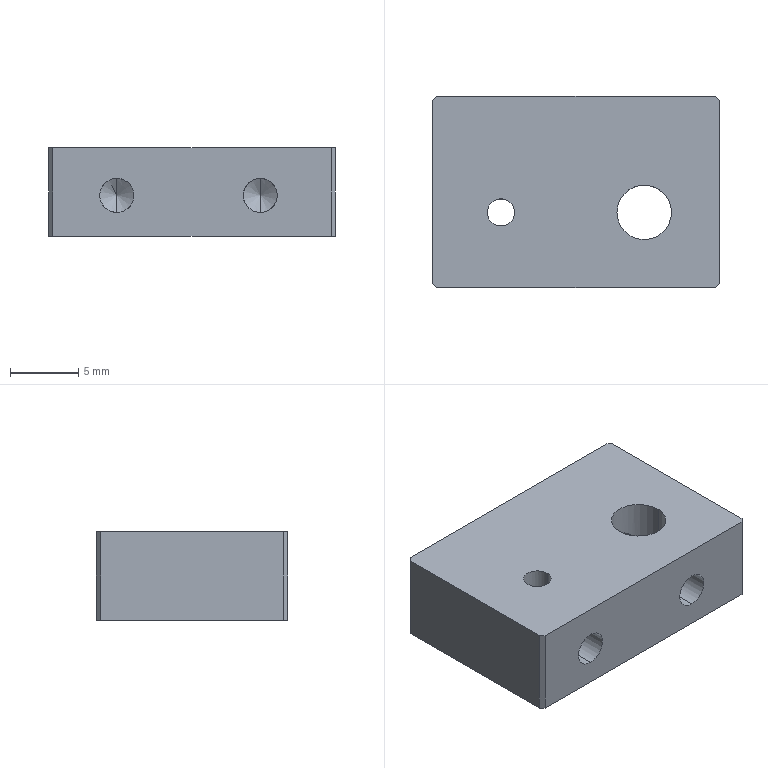Part | NX | features BREP 1 | 1 solid | 26 faces | box 21 x 14 x 6.5 mm | volume 1757 mm3 | cylinder 12 | plane 10 | cone 4 | commonest cylinder face diameters 2.5 x6 2 x4 4 x2
STEP:
#1=CARTESIAN_POINT('',(10.2,-7.,6.5));
#2=VERTEX_POINT('',#1);
#3=CARTESIAN_POINT('',(10.5,-6.7,6.5));
#4=VERTEX_POINT('',#3);
#5=CARTESIAN_POINT('',(10.5,-6.7,6.5));
#6=DIRECTION('',(0.7071,0.7071,0.));
#7=VECTOR('',#6,1000.);
#8=LINE('',#5,#7);
#9=EDGE_CURVE('',#2,#4,#8,.T.);
#10=ORIENTED_EDGE('',*,*,#9,.F.);
#11=CARTESIAN_POINT('',(10.2,-7.,0.));
#12=VERTEX_POINT('',#11);
#13=CARTESIAN_POINT('',(10.2,-7.,6.5));
#14=DIRECTION('',(0.,0.,1.));
#15=VECTOR('',#14,1000.);
#16=LINE('',#13,#15);
#17=EDGE_CURVE('',#12,#2,#16,.T.);
#18=ORIENTED_EDGE('',*,*,#17,.F.);
#19=CARTESIAN_POINT('',(10.5,-6.7,0.));
#20=VERTEX_POINT('',#19);
#21=CARTESIAN_POINT('',(8.6,-8.6,0.));
#22=DIRECTION('',(-0.7071,-0.7071,0.));
#23=VECTOR('',#22,1000.);
#24=LINE('',#21,#23);
#25=EDGE_CURVE('',#20,#12,#24,.T.);
#26=ORIENTED_EDGE('',*,*,#25,.F.);
#27=CARTESIAN_POINT('',(10.5,-6.7,6.5));
#28=DIRECTION('',(0.,0.,-1.));
#29=VECTOR('',#28,1000.);
#30=LINE('',#27,#29);
#31=EDGE_CURVE('',#4,#20,#30,.T.);
#32=ORIENTED_EDGE('',*,*,#31,.F.);
#33=EDGE_LOOP('',(#10,#18,#26,#32));
#34=FACE_BOUND('',#33,.T.);
#35=CARTESIAN_POINT('',(10.5,-6.7,6.5));
#36=DIRECTION('',(-0.7071,0.7071,0.));
#37=DIRECTION('',(0.,0.,-1.));
#38=AXIS2_PLACEMENT_3D('',#35,#36,#37);
#39=PLANE('',#38);
#40=ADVANCED_FACE('',(#34),#39,.F.);
#41=CARTESIAN_POINT('',(10.5,6.7,6.5));
#42=VERTEX_POINT('',#41);
#43=CARTESIAN_POINT('',(10.2,7.,6.5));
#44=VERTEX_POINT('',#43);
#45=CARTESIAN_POINT('',(10.2,7.,6.5));
#46=DIRECTION('',(-0.7071,0.7071,0.));
#47=VECTOR('',#46,1000.);
#48=LINE('',#45,#47);
#49=EDGE_CURVE('',#42,#44,#48,.T.);
#50=ORIENTED_EDGE('',*,*,#49,.F.);
#51=CARTESIAN_POINT('',(10.5,6.7,0.));
#52=VERTEX_POINT('',#51);
#53=CARTESIAN_POINT('',(10.5,6.7,6.5));
#54=DIRECTION('',(0.,0.,1.));
#55=VECTOR('',#54,1000.);
#56=LINE('',#53,#55);
#57=EDGE_CURVE('',#52,#42,#56,.T.);
#58=ORIENTED_EDGE('',*,*,#57,.F.);
#59=CARTESIAN_POINT('',(10.2,7.,0.));
#60=VERTEX_POINT('',#59);
#61=CARTESIAN_POINT('',(8.6,8.6,0.));
#62=DIRECTION('',(0.7071,-0.7071,0.));
#63=VECTOR('',#62,1000.);
#64=LINE('',#61,#63);
#65=EDGE_CURVE('',#60,#52,#64,.T.);
#66=ORIENTED_EDGE('',*,*,#65,.F.);
#67=CARTESIAN_POINT('',(10.2,7.,6.5));
#68=DIRECTION('',(0.,0.,-1.));
#69=VECTOR('',#68,1000.);
#70=LINE('',#67,#69);
#71=EDGE_CURVE('',#44,#60,#70,.T.);
#72=ORIENTED_EDGE('',*,*,#71,.F.);
#73=EDGE_LOOP('',(#50,#58,#66,#72));
#74=FACE_BOUND('',#73,.T.);
#75=CARTESIAN_POINT('',(10.2,7.,6.5));
#76=DIRECTION('',(-0.7071,-0.7071,0.));
#77=DIRECTION('',(0.,0.,-1.));
#78=AXIS2_PLACEMENT_3D('',#75,#76,#77);
#79=PLANE('',#78);
#80=ADVANCED_FACE('',(#74),#79,.F.);
#81=CARTESIAN_POINT('',(-10.2,7.,6.5));
#82=VERTEX_POINT('',#81);
#83=CARTESIAN_POINT('',(-10.5,6.7,6.5));
#84=VERTEX_POINT('',#83);
#85=CARTESIAN_POINT('',(-10.5,6.7,6.5));
#86=DIRECTION('',(-0.7071,-0.7071,0.));
#87=VECTOR('',#86,1000.);
#88=LINE('',#85,#87);
#89=EDGE_CURVE('',#82,#84,#88,.T.);
#90=ORIENTED_EDGE('',*,*,#89,.F.);
#91=CARTESIAN_POINT('',(-10.2,7.,0.));
#92=VERTEX_POINT('',#91);
#93=CARTESIAN_POINT('',(-10.2,7.,6.5));
#94=DIRECTION('',(0.,0.,1.));
#95=VECTOR('',#94,1000.);
#96=LINE('',#93,#95);
#97=EDGE_CURVE('',#92,#82,#96,.T.);
#98=ORIENTED_EDGE('',*,*,#97,.F.);
#99=CARTESIAN_POINT('',(-10.5,6.7,0.));
#100=VERTEX_POINT('',#99);
#101=CARTESIAN_POINT('',(-8.6,8.6,0.));
#102=DIRECTION('',(0.7071,0.7071,0.));
#103=VECTOR('',#102,1000.);
#104=LINE('',#101,#103);
#105=EDGE_CURVE('',#100,#92,#104,.T.);
#106=ORIENTED_EDGE('',*,*,#105,.F.);
#107=CARTESIAN_POINT('',(-10.5,6.7,6.5));
#108=DIRECTION('',(0.,0.,-1.));
#109=VECTOR('',#108,1000.);
#110=LINE('',#107,#109);
#111=EDGE_CURVE('',#84,#100,#110,.T.);
#112=ORIENTED_EDGE('',*,*,#111,.F.);
#113=EDGE_LOOP('',(#90,#98,#106,#112));
#114=FACE_BOUND('',#113,.T.);
#115=CARTESIAN_POINT('',(-10.5,6.7,6.5));
#116=DIRECTION('',(0.7071,-0.7071,0.));
#117=DIRECTION('',(0.,0.,-1.));
#118=AXIS2_PLACEMENT_3D('',#115,#116,#117);
#119=PLANE('',#118);
#120=ADVANCED_FACE('',(#114),#119,.F.);
#121=CARTESIAN_POINT('',(-10.5,-6.7,6.5));
#122=VERTEX_POINT('',#121);
#123=CARTESIAN_POINT('',(-10.2,-7.,6.5));
#124=VERTEX_POINT('',#123);
#125=CARTESIAN_POINT('',(-10.2,-7.,6.5));
#126=DIRECTION('',(0.7071,-0.7071,0.));
#127=VECTOR('',#126,1000.);
#128=LINE('',#125,#127);
#129=EDGE_CURVE('',#122,#124,#128,.T.);
#130=ORIENTED_EDGE('',*,*,#129,.F.);
#131=CARTESIAN_POINT('',(-10.5,-6.7,0.));
#132=VERTEX_POINT('',#131);
#133=CARTESIAN_POINT('',(-10.5,-6.7,6.5));
#134=DIRECTION('',(0.,0.,1.));
#135=VECTOR('',#134,1000.);
#136=LINE('',#133,#135);
#137=EDGE_CURVE('',#132,#122,#136,.T.);
#138=ORIENTED_EDGE('',*,*,#137,.F.);
#139=CARTESIAN_POINT('',(-10.2,-7.,0.));
#140=VERTEX_POINT('',#139);
#141=CARTESIAN_POINT('',(-8.6,-8.6,0.));
#142=DIRECTION('',(-0.7071,0.7071,0.));
#143=VECTOR('',#142,1000.);
#144=LINE('',#141,#143);
#145=EDGE_CURVE('',#140,#132,#144,.T.);
#146=ORIENTED_EDGE('',*,*,#145,.F.);
#147=CARTESIAN_POINT('',(-10.2,-7.,6.5));
#148=DIRECTION('',(0.,0.,-1.));
#149=VECTOR('',#148,1000.);
#150=LINE('',#147,#149);
#151=EDGE_CURVE('',#124,#140,#150,.T.);
#152=ORIENTED_EDGE('',*,*,#151,.F.);
#153=EDGE_LOOP('',(#130,#138,#146,#152));
#154=FACE_BOUND('',#153,.T.);
#155=CARTESIAN_POINT('',(-10.2,-7.,6.5));
#156=DIRECTION('',(0.7071,0.7071,0.));
#157=DIRECTION('',(0.,0.,-1.));
#158=AXIS2_PLACEMENT_3D('',#155,#156,#157);
#159=PLANE('',#158);
#160=ADVANCED_FACE('',(#154),#159,.F.);
#161=CARTESIAN_POINT('',(5.,0.5,4.25));
#162=VERTEX_POINT('',#161);
#163=CARTESIAN_POINT('',(5.,1.251,3.));
#164=VERTEX_POINT('',#163);
#165=CARTESIAN_POINT('',(5.,0.5,4.25));
#166=DIRECTION('',(0.,-0.515,0.8572));
#167=VECTOR('',#166,1000.);
#168=LINE('',#165,#167);
#169=EDGE_CURVE('',#162,#164,#168,.F.);
#170=ORIENTED_EDGE('',*,*,#169,.T.);
#171=CARTESIAN_POINT('',(5.,0.5,1.75));
#172=VERTEX_POINT('',#171);
#173=CARTESIAN_POINT('',(5.,0.5,1.75));
#174=DIRECTION('',(0.,-0.515,-0.8572));
#175=VECTOR('',#174,1000.);
#176=LINE('',#173,#175);
#177=EDGE_CURVE('',#172,#164,#176,.F.);
#178=ORIENTED_EDGE('',*,*,#177,.F.);
#179=CARTESIAN_POINT('',(5.,0.5,3.));
#180=DIRECTION('',(0.,-1.,0.));
#181=DIRECTION('',(0.,0.,-1.));
#182=AXIS2_PLACEMENT_3D('',#179,#180,#181);
#183=CIRCLE('',#182,1.25);
#184=EDGE_CURVE('',#172,#162,#183,.T.);
#185=ORIENTED_EDGE('',*,*,#184,.T.);
#186=EDGE_LOOP('',(#170,#178,#185));
#187=FACE_BOUND('',#186,.T.);
#188=CARTESIAN_POINT('',(5.,0.5,3.));
#189=DIRECTION('',(0.,-1.,0.));
#190=DIRECTION('',(0.,0.,-1.));
#191=AXIS2_PLACEMENT_3D('',#188,#189,#190);
#192=CONICAL_SURFACE('',#191,1.25,1.03);
#193=ADVANCED_FACE('',(#187),#192,.F.);
#194=CARTESIAN_POINT('',(5.,0.5,4.25));
#195=CARTESIAN_POINT('',(4.84,0.5,4.25));
#196=CARTESIAN_POINT('',(4.56,0.4617,4.19));
#197=CARTESIAN_POINT('',(4.324,0.3832,4.054));
#198=CARTESIAN_POINT('',(4.169,0.3251,3.954));
#199=CARTESIAN_POINT('',(3.974,0.218,3.718));
#200=CARTESIAN_POINT('',(3.979,0.2199,3.723));
#201=CARTESIAN_POINT('',(3.889,0.1639,3.58));
#202=CARTESIAN_POINT('',(3.807,0.1064,3.399));
#203=CARTESIAN_POINT('',(3.704,0.02524,3.001));
#204=CARTESIAN_POINT('',(3.807,0.1061,2.602));
#205=CARTESIAN_POINT('',(3.888,0.1634,2.422));
#206=CARTESIAN_POINT('',(3.979,0.2195,2.278));
#207=CARTESIAN_POINT('',(3.974,0.2185,2.28));
#208=CARTESIAN_POINT('',(4.174,0.3265,2.043));
#209=CARTESIAN_POINT('',(4.282,0.3685,1.974));
#210=CARTESIAN_POINT('',(4.585,0.4703,1.794));
#211=CARTESIAN_POINT('',(4.84,0.5,1.75));
#212=CARTESIAN_POINT('',(5.,0.5,1.75));
#213=B_SPLINE_CURVE_WITH_KNOTS('',3,(#194,#195,#196,#197,#198,#199,#200,#201,#202,#203,#204,#205,#206,#207,#208,#209,#210,#211,#212),.UNSPECIFIED.,.F.,.F.,(4,1,1,1,1,1,1,1,1,1,1,1,1,1,1,1,4),(0.,0.125,0.1875,0.25,0.2812,0.3125,0.3438,0.375,0.5,0.625,0.6562,0.6875,0.7188,0.75,0.8125,0.875,1.),.UNSPECIFIED.);
#214=EDGE_CURVE('',#162,#172,#213,.T.);
#215=ORIENTED_EDGE('',*,*,#214,.T.);
#216=CARTESIAN_POINT('',(5.,0.5,3.));
#217=DIRECTION('',(0.,-1.,0.));
#218=DIRECTION('',(0.,0.,-1.));
#219=AXIS2_PLACEMENT_3D('',#216,#217,#218);
#220=CIRCLE('',#219,1.25);
#221=EDGE_CURVE('',#162,#172,#220,.T.);
#222=ORIENTED_EDGE('',*,*,#221,.F.);
#223=EDGE_LOOP('',(#215,#222));
#224=FACE_BOUND('',#223,.T.);
#225=CARTESIAN_POINT('',(5.,-7.,3.));
#226=DIRECTION('',(0.,-1.,0.));
#227=DIRECTION('',(0.,0.,-1.));
#228=AXIS2_PLACEMENT_3D('',#225,#226,#227);
#229=CYLINDRICAL_SURFACE('',#228,1.25);
#230=ADVANCED_FACE('',(#224),#229,.F.);
#231=CARTESIAN_POINT('',(5.,0.5,1.75));
#232=CARTESIAN_POINT('',(5.16,0.5,1.75));
#233=CARTESIAN_POINT('',(5.44,0.4614,1.811));
#234=CARTESIAN_POINT('',(5.675,0.3833,1.946));
#235=CARTESIAN_POINT('',(5.832,0.3242,2.048));
#236=CARTESIAN_POINT('',(6.024,0.2193,2.279));
#237=CARTESIAN_POINT('',(6.021,0.2195,2.278));
#238=CARTESIAN_POINT('',(6.111,0.1638,2.421));
#239=CARTESIAN_POINT('',(6.192,0.1068,2.6));
#240=CARTESIAN_POINT('',(6.296,0.02501,3.));
#241=CARTESIAN_POINT('',(6.193,0.1064,3.399));
#242=CARTESIAN_POINT('',(6.112,0.1635,3.578));
#243=CARTESIAN_POINT('',(6.021,0.2195,3.722));
#244=CARTESIAN_POINT('',(6.026,0.2185,3.72));
#245=CARTESIAN_POINT('',(5.826,0.3266,3.957));
#246=CARTESIAN_POINT('',(5.717,0.3689,4.026));
#247=CARTESIAN_POINT('',(5.415,0.4702,4.206));
#248=CARTESIAN_POINT('',(5.16,0.5,4.25));
#249=CARTESIAN_POINT('',(5.,0.5,4.25));
#250=B_SPLINE_CURVE_WITH_KNOTS('',3,(#231,#232,#233,#234,#235,#236,#237,#238,#239,#240,#241,#242,#243,#244,#245,#246,#247,#248,#249),.UNSPECIFIED.,.F.,.F.,(4,1,1,1,1,1,1,1,1,1,1,1,1,1,1,1,4),(0.,0.125,0.1875,0.25,0.2812,0.3125,0.3438,0.375,0.5,0.625,0.6562,0.6875,0.7188,0.75,0.8125,0.875,1.),.UNSPECIFIED.);
#251=EDGE_CURVE('',#172,#162,#250,.T.);
#252=ORIENTED_EDGE('',*,*,#251,.T.);
#253=ORIENTED_EDGE('',*,*,#184,.F.);
#254=EDGE_LOOP('',(#252,#253));
#255=FACE_BOUND('',#254,.T.);
#256=CARTESIAN_POINT('',(5.,-7.,3.));
#257=DIRECTION('',(0.,-1.,0.));
#258=DIRECTION('',(0.,0.,-1.));
#259=AXIS2_PLACEMENT_3D('',#256,#257,#258);
#260=CYLINDRICAL_SURFACE('',#259,1.25);
#261=ADVANCED_FACE('',(#255),#260,.F.);
#262=CARTESIAN_POINT('',(5.,-3.5,4.25));
#263=VERTEX_POINT('',#262);
#264=CARTESIAN_POINT('',(5.,-7.,4.25));
#265=VERTEX_POINT('',#264);
#266=CARTESIAN_POINT('',(5.,-7.,4.25));
#267=DIRECTION('',(0.,-1.,0.));
#268=VECTOR('',#267,1000.);
#269=LINE('',#266,#268);
#270=EDGE_CURVE('',#263,#265,#269,.T.);
#271=ORIENTED_EDGE('',*,*,#270,.F.);
#272=CARTESIAN_POINT('',(5.,-3.5,1.75));
#273=VERTEX_POINT('',#272);
#274=CARTESIAN_POINT('',(5.,-3.5,4.25));
#275=CARTESIAN_POINT('',(5.16,-3.5,4.25));
#276=CARTESIAN_POINT('',(5.44,-3.462,4.19));
#277=CARTESIAN_POINT('',(5.676,-3.383,4.054));
#278=CARTESIAN_POINT('',(5.831,-3.325,3.954));
#279=CARTESIAN_POINT('',(6.026,-3.218,3.718));
#280=CARTESIAN_POINT('',(6.021,-3.22,3.723));
#281=CARTESIAN_POINT('',(6.111,-3.164,3.58));
#282=CARTESIAN_POINT('',(6.193,-3.106,3.399));
#283=CARTESIAN_POINT('',(6.296,-3.025,3.001));
#284=CARTESIAN_POINT('',(6.193,-3.106,2.602));
#285=CARTESIAN_POINT('',(6.112,-3.163,2.422));
#286=CARTESIAN_POINT('',(6.021,-3.22,2.278));
#287=CARTESIAN_POINT('',(6.026,-3.218,2.28));
#288=CARTESIAN_POINT('',(5.826,-3.327,2.043));
#289=CARTESIAN_POINT('',(5.718,-3.369,1.974));
#290=CARTESIAN_POINT('',(5.415,-3.47,1.794));
#291=CARTESIAN_POINT('',(5.16,-3.5,1.75));
#292=CARTESIAN_POINT('',(5.,-3.5,1.75));
#293=B_SPLINE_CURVE_WITH_KNOTS('',3,(#274,#275,#276,#277,#278,#279,#280,#281,#282,#283,#284,#285,#286,#287,#288,#289,#290,#291,#292),.UNSPECIFIED.,.F.,.F.,(4,1,1,1,1,1,1,1,1,1,1,1,1,1,1,1,4),(0.,0.125,0.1875,0.25,0.2812,0.3125,0.3438,0.375,0.5,0.625,0.6562,0.6875,0.7188,0.75,0.8125,0.875,1.),.UNSPECIFIED.);
#294=EDGE_CURVE('',#263,#273,#293,.T.);
#295=ORIENTED_EDGE('',*,*,#294,.T.);
#296=CARTESIAN_POINT('',(5.,-7.,1.75));
#297=VERTEX_POINT('',#296);
#298=CARTESIAN_POINT('',(5.,-7.,1.75));
#299=DIRECTION('',(0.,-1.,0.));
#300=VECTOR('',#299,1000.);
#301=LINE('',#298,#300);
#302=EDGE_CURVE('',#273,#297,#301,.T.);
#303=ORIENTED_EDGE('',*,*,#302,.T.);
#304=CARTESIAN_POINT('',(5.,-7.,3.));
#305=DIRECTION('',(0.,-1.,0.));
#306=DIRECTION('',(0.,0.,-1.));
#307=AXIS2_PLACEMENT_3D('',#304,#305,#306);
#308=CIRCLE('',#307,1.25);
#309=EDGE_CURVE('',#297,#265,#308,.T.);
#310=ORIENTED_EDGE('',*,*,#309,.T.);
#311=EDGE_LOOP('',(#271,#295,#303,#310));
#312=FACE_BOUND('',#311,.T.);
#313=CARTESIAN_POINT('',(5.,-7.,3.));
#314=DIRECTION('',(0.,-1.,0.));
#315=DIRECTION('',(0.,0.,-1.));
#316=AXIS2_PLACEMENT_3D('',#313,#314,#315);
#317=CYLINDRICAL_SURFACE('',#316,1.25);
#318=ADVANCED_FACE('',(#312),#317,.F.);
#319=CARTESIAN_POINT('',(-5.5,0.5,4.25));
#320=VERTEX_POINT('',#319);
#321=CARTESIAN_POINT('',(-5.5,-0.5,4.25));
#322=VERTEX_POINT('',#321);
#323=CARTESIAN_POINT('',(-5.5,-7.,4.25));
#324=DIRECTION('',(0.,-1.,0.));
#325=VECTOR('',#324,1000.);
#326=LINE('',#323,#325);
#327=EDGE_CURVE('',#320,#322,#326,.T.);
#328=ORIENTED_EDGE('',*,*,#327,.F.);
#329=CARTESIAN_POINT('',(-5.5,0.5,1.75));
#330=VERTEX_POINT('',#329);
#331=CARTESIAN_POINT('',(-5.5,0.5,3.));
#332=DIRECTION('',(0.,-1.,0.));
#333=DIRECTION('',(0.,0.,-1.));
#334=AXIS2_PLACEMENT_3D('',#331,#332,#333);
#335=CIRCLE('',#334,1.25);
#336=EDGE_CURVE('',#330,#320,#335,.T.);
#337=ORIENTED_EDGE('',*,*,#336,.F.);
#338=CARTESIAN_POINT('',(-5.5,-0.5,1.75));
#339=VERTEX_POINT('',#338);
#340=CARTESIAN_POINT('',(-5.5,-7.,1.75));
#341=DIRECTION('',(0.,-1.,0.));
#342=VECTOR('',#341,1000.);
#343=LINE('',#340,#342);
#344=EDGE_CURVE('',#339,#330,#343,.F.);
#345=ORIENTED_EDGE('',*,*,#344,.F.);
#346=CARTESIAN_POINT('',(-4.5,-1.5,2.25));
#347=VERTEX_POINT('',#346);
#348=CARTESIAN_POINT('',(-5.5,-0.5,1.75));
#349=CARTESIAN_POINT('',(-5.228,-0.5,1.75));
#350=CARTESIAN_POINT('',(-4.71,-0.7266,1.947));
#351=CARTESIAN_POINT('',(-4.5,-1.242,2.25));
#352=CARTESIAN_POINT('',(-4.5,-1.5,2.25));
#353=B_SPLINE_CURVE_WITH_KNOTS('',3,(#348,#349,#350,#351,#352),.UNSPECIFIED.,.F.,.F.,(4,1,4),(0.,0.5,1.),.UNSPECIFIED.);
#354=EDGE_CURVE('',#339,#347,#353,.T.);
#355=ORIENTED_EDGE('',*,*,#354,.T.);
#356=CARTESIAN_POINT('',(-5.5,-2.5,1.75));
#357=VERTEX_POINT('',#356);
#358=CARTESIAN_POINT('',(-4.5,-1.5,2.25));
#359=CARTESIAN_POINT('',(-4.5,-1.757,2.25));
#360=CARTESIAN_POINT('',(-4.71,-2.273,1.947));
#361=CARTESIAN_POINT('',(-5.227,-2.5,1.75));
#362=CARTESIAN_POINT('',(-5.5,-2.5,1.75));
#363=B_SPLINE_CURVE_WITH_KNOTS('',3,(#358,#359,#360,#361,#362),.UNSPECIFIED.,.F.,.F.,(4,1,4),(0.,0.5,1.),.UNSPECIFIED.);
#364=EDGE_CURVE('',#347,#357,#363,.T.);
#365=ORIENTED_EDGE('',*,*,#364,.T.);
#366=CARTESIAN_POINT('',(-5.5,-7.,1.75));
#367=VERTEX_POINT('',#366);
#368=CARTESIAN_POINT('',(-5.5,-7.,1.75));
#369=DIRECTION('',(0.,-1.,0.));
#370=VECTOR('',#369,1000.);
#371=LINE('',#368,#370);
#372=EDGE_CURVE('',#357,#367,#371,.T.);
#373=ORIENTED_EDGE('',*,*,#372,.T.);
#374=CARTESIAN_POINT('',(-5.5,-7.,4.25));
#375=VERTEX_POINT('',#374);
#376=CARTESIAN_POINT('',(-5.5,-7.,3.));
#377=DIRECTION('',(0.,-1.,0.));
#378=DIRECTION('',(0.,0.,-1.));
#379=AXIS2_PLACEMENT_3D('',#376,#377,#378);
#380=CIRCLE('',#379,1.25);
#381=EDGE_CURVE('',#367,#375,#380,.T.);
#382=ORIENTED_EDGE('',*,*,#381,.T.);
#383=CARTESIAN_POINT('',(-5.5,-2.5,4.25));
#384=VERTEX_POINT('',#383);
#385=CARTESIAN_POINT('',(-5.5,-7.,4.25));
#386=DIRECTION('',(0.,-1.,0.));
#387=VECTOR('',#386,1000.);
#388=LINE('',#385,#387);
#389=EDGE_CURVE('',#375,#384,#388,.F.);
#390=ORIENTED_EDGE('',*,*,#389,.T.);
#391=CARTESIAN_POINT('',(-4.5,-1.5,3.75));
#392=VERTEX_POINT('',#391);
#393=CARTESIAN_POINT('',(-5.5,-2.5,4.25));
#394=CARTESIAN_POINT('',(-5.228,-2.5,4.25));
#395=CARTESIAN_POINT('',(-4.71,-2.273,4.053));
#396=CARTESIAN_POINT('',(-4.5,-1.758,3.75));
#397=CARTESIAN_POINT('',(-4.5,-1.5,3.75));
#398=B_SPLINE_CURVE_WITH_KNOTS('',3,(#393,#394,#395,#396,#397),.UNSPECIFIED.,.F.,.F.,(4,1,4),(0.,0.5,1.),.UNSPECIFIED.);
#399=EDGE_CURVE('',#384,#392,#398,.T.);
#400=ORIENTED_EDGE('',*,*,#399,.T.);
#401=CARTESIAN_POINT('',(-4.5,-1.5,3.75));
#402=CARTESIAN_POINT('',(-4.5,-1.243,3.75));
#403=CARTESIAN_POINT('',(-4.71,-0.7266,4.053));
#404=CARTESIAN_POINT('',(-5.227,-0.5,4.25));
#405=CARTESIAN_POINT('',(-5.5,-0.5,4.25));
#406=B_SPLINE_CURVE_WITH_KNOTS('',3,(#401,#402,#403,#404,#405),.UNSPECIFIED.,.F.,.F.,(4,1,4),(0.,0.5,1.),.UNSPECIFIED.);
#407=EDGE_CURVE('',#392,#322,#406,.T.);
#408=ORIENTED_EDGE('',*,*,#407,.T.);
#409=EDGE_LOOP('',(#328,#337,#345,#355,#365,#373,#382,#390,#400,#408));
#410=FACE_BOUND('',#409,.T.);
#411=CARTESIAN_POINT('',(-5.5,-7.,3.));
#412=DIRECTION('',(0.,-1.,0.));
#413=DIRECTION('',(0.,0.,-1.));
#414=AXIS2_PLACEMENT_3D('',#411,#412,#413);
#415=CYLINDRICAL_SURFACE('',#414,1.25);
#416=ADVANCED_FACE('',(#410),#415,.F.);
#417=CARTESIAN_POINT('',(-5.5,1.251,3.));
#418=VERTEX_POINT('',#417);
#419=CARTESIAN_POINT('',(-5.5,0.5,4.25));
#420=DIRECTION('',(0.,-0.515,0.8572));
#421=VECTOR('',#420,1000.);
#422=LINE('',#419,#421);
#423=EDGE_CURVE('',#320,#418,#422,.F.);
#424=ORIENTED_EDGE('',*,*,#423,.T.);
#425=CARTESIAN_POINT('',(-5.5,0.5,1.75));
#426=DIRECTION('',(0.,-0.515,-0.8572));
#427=VECTOR('',#426,1000.);
#428=LINE('',#425,#427);
#429=EDGE_CURVE('',#330,#418,#428,.F.);
#430=ORIENTED_EDGE('',*,*,#429,.F.);
#431=ORIENTED_EDGE('',*,*,#336,.T.);
#432=EDGE_LOOP('',(#424,#430,#431));
#433=FACE_BOUND('',#432,.T.);
#434=CARTESIAN_POINT('',(-5.5,0.5,3.));
#435=DIRECTION('',(0.,-1.,0.));
#436=DIRECTION('',(0.,0.,-1.));
#437=AXIS2_PLACEMENT_3D('',#434,#435,#436);
#438=CONICAL_SURFACE('',#437,1.25,1.03);
#439=ADVANCED_FACE('',(#433),#438,.F.);
#440=ORIENTED_EDGE('',*,*,#251,.F.);
#441=ORIENTED_EDGE('',*,*,#214,.F.);
#442=EDGE_LOOP('',(#440,#441));
#443=FACE_BOUND('',#442,.T.);
#444=CARTESIAN_POINT('',(7.,-1.5,6.5));
#445=VERTEX_POINT('',#444);
#446=CARTESIAN_POINT('',(7.,-1.5,0.));
#447=VERTEX_POINT('',#446);
#448=CARTESIAN_POINT('',(7.,-1.5,6.5));
#449=DIRECTION('',(0.,0.,-1.));
#450=VECTOR('',#449,1000.);
#451=LINE('',#448,#450);
#452=EDGE_CURVE('',#445,#447,#451,.T.);
#453=ORIENTED_EDGE('',*,*,#452,.F.);
#454=CARTESIAN_POINT('',(3.,-1.5,6.5));
#455=VERTEX_POINT('',#454);
#456=CARTESIAN_POINT('',(5.,-1.5,6.5));
#457=DIRECTION('',(0.,0.,1.));
#458=DIRECTION('',(1.,0.,0.));
#459=AXIS2_PLACEMENT_3D('',#456,#457,#458);
#460=CIRCLE('',#459,2.);
#461=EDGE_CURVE('',#445,#455,#460,.T.);
#462=ORIENTED_EDGE('',*,*,#461,.T.);
#463=CARTESIAN_POINT('',(3.,-1.5,0.));
#464=VERTEX_POINT('',#463);
#465=CARTESIAN_POINT('',(3.,-1.5,6.5));
#466=DIRECTION('',(0.,0.,-1.));
#467=VECTOR('',#466,1000.);
#468=LINE('',#465,#467);
#469=EDGE_CURVE('',#455,#464,#468,.T.);
#470=ORIENTED_EDGE('',*,*,#469,.T.);
#471=CARTESIAN_POINT('',(5.,-1.5,0.));
#472=DIRECTION('',(0.,0.,1.));
#473=DIRECTION('',(1.,0.,0.));
#474=AXIS2_PLACEMENT_3D('',#471,#472,#473);
#475=CIRCLE('',#474,2.);
#476=EDGE_CURVE('',#447,#464,#475,.T.);
#477=ORIENTED_EDGE('',*,*,#476,.F.);
#478=EDGE_LOOP('',(#453,#462,#470,#477));
#479=FACE_BOUND('',#478,.T.);
#480=CARTESIAN_POINT('',(5.,-1.5,6.5));
#481=DIRECTION('',(0.,0.,-1.));
#482=DIRECTION('',(-1.,0.,0.));
#483=AXIS2_PLACEMENT_3D('',#480,#481,#482);
#484=CYLINDRICAL_SURFACE('',#483,2.);
#485=ADVANCED_FACE('',(#443,#479),#484,.F.);
#486=CARTESIAN_POINT('',(-4.5,-1.5,0.));
#487=VERTEX_POINT('',#486);
#488=CARTESIAN_POINT('',(-4.5,-1.5,6.5));
#489=DIRECTION('',(0.,0.,-1.));
#490=VECTOR('',#489,1000.);
#491=LINE('',#488,#490);
#492=EDGE_CURVE('',#347,#487,#491,.T.);
#493=ORIENTED_EDGE('',*,*,#492,.F.);
#494=ORIENTED_EDGE('',*,*,#354,.F.);
#495=CARTESIAN_POINT('',(-6.5,-1.5,2.25));
#496=VERTEX_POINT('',#495);
#497=CARTESIAN_POINT('',(-5.5,-0.5,1.75));
#498=CARTESIAN_POINT('',(-5.765,-0.5,1.75));
#499=CARTESIAN_POINT('',(-6.168,-0.689,1.903));
#500=CARTESIAN_POINT('',(-6.439,-1.083,2.166));
#501=CARTESIAN_POINT('',(-6.5,-1.382,2.25));
#502=CARTESIAN_POINT('',(-6.5,-1.5,2.25));
#503=B_SPLINE_CURVE_WITH_KNOTS('',3,(#497,#498,#499,#500,#501,#502),.UNSPECIFIED.,.F.,.F.,(4,1,1,4),(0.,0.5,0.75,1.),.UNSPECIFIED.);
#504=EDGE_CURVE('',#496,#339,#503,.F.);
#505=ORIENTED_EDGE('',*,*,#504,.F.);
#506=CARTESIAN_POINT('',(-6.5,-1.5,0.));
#507=VERTEX_POINT('',#506);
#508=CARTESIAN_POINT('',(-6.5,-1.5,6.5));
#509=DIRECTION('',(0.,0.,-1.));
#510=VECTOR('',#509,1000.);
#511=LINE('',#508,#510);
#512=EDGE_CURVE('',#496,#507,#511,.T.);
#513=ORIENTED_EDGE('',*,*,#512,.T.);
#514=CARTESIAN_POINT('',(-5.5,-1.5,0.));
#515=DIRECTION('',(0.,0.,1.));
#516=DIRECTION('',(1.,0.,0.));
#517=AXIS2_PLACEMENT_3D('',#514,#515,#516);
#518=CIRCLE('',#517,1.);
#519=EDGE_CURVE('',#487,#507,#518,.T.);
#520=ORIENTED_EDGE('',*,*,#519,.F.);
#521=EDGE_LOOP('',(#493,#494,#505,#513,#520));
#522=FACE_BOUND('',#521,.T.);
#523=CARTESIAN_POINT('',(-5.5,-1.5,6.5));
#524=DIRECTION('',(0.,0.,-1.));
#525=DIRECTION('',(-1.,0.,0.));
#526=AXIS2_PLACEMENT_3D('',#523,#524,#525);
#527=CYLINDRICAL_SURFACE('',#526,1.);
#528=ADVANCED_FACE('',(#522),#527,.F.);
#529=CARTESIAN_POINT('',(-10.5,-7.,6.5));
#530=DIRECTION('',(1.,0.,0.));
#531=VECTOR('',#530,1000.);
#532=LINE('',#529,#531);
#533=EDGE_CURVE('',#124,#2,#532,.T.);
#534=ORIENTED_EDGE('',*,*,#533,.F.);
#535=ORIENTED_EDGE('',*,*,#151,.T.);
#536=CARTESIAN_POINT('',(-10.5,-7.,0.));
#537=DIRECTION('',(1.,0.,0.));
#538=VECTOR('',#537,1000.);
#539=LINE('',#536,#538);
#540=EDGE_CURVE('',#140,#12,#539,.T.);
#541=ORIENTED_EDGE('',*,*,#540,.T.);
#542=ORIENTED_EDGE('',*,*,#17,.T.);
#543=EDGE_LOOP('',(#534,#535,#541,#542));
#544=FACE_BOUND('',#543,.T.);
#545=ORIENTED_EDGE('',*,*,#381,.F.);
#546=CARTESIAN_POINT('',(-5.5,-7.,3.));
#547=DIRECTION('',(0.,-1.,0.));
#548=DIRECTION('',(0.,0.,-1.));
#549=AXIS2_PLACEMENT_3D('',#546,#547,#548);
#550=CIRCLE('',#549,1.25);
#551=EDGE_CURVE('',#375,#367,#550,.T.);
#552=ORIENTED_EDGE('',*,*,#551,.F.);
#553=EDGE_LOOP('',(#545,#552));
#554=FACE_BOUND('',#553,.T.);
#555=ORIENTED_EDGE('',*,*,#309,.F.);
#556=CARTESIAN_POINT('',(5.,-7.,3.));
#557=DIRECTION('',(0.,-1.,0.));
#558=DIRECTION('',(0.,0.,-1.));
#559=AXIS2_PLACEMENT_3D('',#556,#557,#558);
#560=CIRCLE('',#559,1.25);
#561=EDGE_CURVE('',#265,#297,#560,.T.);
#562=ORIENTED_EDGE('',*,*,#561,.F.);
#563=EDGE_LOOP('',(#555,#562));
#564=FACE_BOUND('',#563,.T.);
#565=CARTESIAN_POINT('',(-10.5,-7.,6.5));
#566=DIRECTION('',(0.,1.,0.));
#567=DIRECTION('',(0.,0.,1.));
#568=AXIS2_PLACEMENT_3D('',#565,#566,#567);
#569=PLANE('',#568);
#570=ADVANCED_FACE('',(#544,#554,#564),#569,.F.);
#571=CARTESIAN_POINT('',(-10.5,-7.,0.));
#572=DIRECTION('',(0.,-1.,0.));
#573=VECTOR('',#572,1000.);
#574=LINE('',#571,#573);
#575=EDGE_CURVE('',#100,#132,#574,.T.);
#576=ORIENTED_EDGE('',*,*,#575,.T.);
#577=ORIENTED_EDGE('',*,*,#137,.T.);
#578=CARTESIAN_POINT('',(-10.5,-7.,6.5));
#579=DIRECTION('',(0.,-1.,0.));
#580=VECTOR('',#579,1000.);
#581=LINE('',#578,#580);
#582=EDGE_CURVE('',#84,#122,#581,.T.);
#583=ORIENTED_EDGE('',*,*,#582,.F.);
#584=ORIENTED_EDGE('',*,*,#111,.T.);
#585=EDGE_LOOP('',(#576,#577,#583,#584));
#586=FACE_BOUND('',#585,.T.);
#587=CARTESIAN_POINT('',(-10.5,-7.,6.5));
#588=DIRECTION('',(1.,0.,0.));
#589=DIRECTION('',(0.,0.,-1.));
#590=AXIS2_PLACEMENT_3D('',#587,#588,#589);
#591=PLANE('',#590);
#592=ADVANCED_FACE('',(#586),#591,.F.);
#593=CARTESIAN_POINT('',(-10.5,7.,0.));
#594=DIRECTION('',(-1.,0.,0.));
#595=VECTOR('',#594,1000.);
#596=LINE('',#593,#595);
#597=EDGE_CURVE('',#60,#92,#596,.T.);
#598=ORIENTED_EDGE('',*,*,#597,.T.);
#599=ORIENTED_EDGE('',*,*,#97,.T.);
#600=CARTESIAN_POINT('',(-10.5,7.,6.5));
#601=DIRECTION('',(-1.,0.,0.));
#602=VECTOR('',#601,1000.);
#603=LINE('',#600,#602);
#604=EDGE_CURVE('',#44,#82,#603,.T.);
#605=ORIENTED_EDGE('',*,*,#604,.F.);
#606=ORIENTED_EDGE('',*,*,#71,.T.);
#607=EDGE_LOOP('',(#598,#599,#605,#606));
#608=FACE_BOUND('',#607,.T.);
#609=CARTESIAN_POINT('',(-10.5,7.,6.5));
#610=DIRECTION('',(0.,-1.,0.));
#611=DIRECTION('',(0.,0.,-1.));
#612=AXIS2_PLACEMENT_3D('',#609,#610,#611);
#613=PLANE('',#612);
#614=ADVANCED_FACE('',(#608),#613,.F.);
#615=CARTESIAN_POINT('',(10.5,-7.,0.));
#616=DIRECTION('',(0.,1.,0.));
#617=VECTOR('',#616,1000.);
#618=LINE('',#615,#617);
#619=EDGE_CURVE('',#20,#52,#618,.T.);
#620=ORIENTED_EDGE('',*,*,#619,.T.);
#621=ORIENTED_EDGE('',*,*,#57,.T.);
#622=CARTESIAN_POINT('',(10.5,-7.,6.5));
#623=DIRECTION('',(0.,1.,0.));
#624=VECTOR('',#623,1000.);
#625=LINE('',#622,#624);
#626=EDGE_CURVE('',#4,#42,#625,.T.);
#627=ORIENTED_EDGE('',*,*,#626,.F.);
#628=ORIENTED_EDGE('',*,*,#31,.T.);
#629=EDGE_LOOP('',(#620,#621,#627,#628));
#630=FACE_BOUND('',#629,.T.);
#631=CARTESIAN_POINT('',(10.5,-7.,6.5));
#632=DIRECTION('',(-1.,0.,0.));
#633=DIRECTION('',(0.,0.,1.));
#634=AXIS2_PLACEMENT_3D('',#631,#632,#633);
#635=PLANE('',#634);
#636=ADVANCED_FACE('',(#630),#635,.F.);
#637=CARTESIAN_POINT('',(5.,-1.5,0.));
#638=DIRECTION('',(0.,0.,1.));
#639=DIRECTION('',(1.,0.,0.));
#640=AXIS2_PLACEMENT_3D('',#637,#638,#639);
#641=CIRCLE('',#640,2.);
#642=EDGE_CURVE('',#464,#447,#641,.T.);
#643=ORIENTED_EDGE('',*,*,#642,.T.);
#644=ORIENTED_EDGE('',*,*,#476,.T.);
#645=EDGE_LOOP('',(#643,#644));
#646=FACE_BOUND('',#645,.T.);
#647=ORIENTED_EDGE('',*,*,#540,.F.);
#648=ORIENTED_EDGE('',*,*,#145,.T.);
#649=ORIENTED_EDGE('',*,*,#575,.F.);
#650=ORIENTED_EDGE('',*,*,#105,.T.);
#651=ORIENTED_EDGE('',*,*,#597,.F.);
#652=ORIENTED_EDGE('',*,*,#65,.T.);
#653=ORIENTED_EDGE('',*,*,#619,.F.);
#654=ORIENTED_EDGE('',*,*,#25,.T.);
#655=EDGE_LOOP('',(#647,#648,#649,#650,#651,#652,#653,#654));
#656=FACE_BOUND('',#655,.T.);
#657=CARTESIAN_POINT('',(-5.5,-1.5,0.));
#658=DIRECTION('',(0.,0.,1.));
#659=DIRECTION('',(1.,0.,0.));
#660=AXIS2_PLACEMENT_3D('',#657,#658,#659);
#661=CIRCLE('',#660,1.);
#662=EDGE_CURVE('',#507,#487,#661,.T.);
#663=ORIENTED_EDGE('',*,*,#662,.T.);
#664=ORIENTED_EDGE('',*,*,#519,.T.);
#665=EDGE_LOOP('',(#663,#664));
#666=FACE_BOUND('',#665,.T.);
#667=CARTESIAN_POINT('',(0.,0.,0.));
#668=DIRECTION('',(0.,0.,-1.));
#669=DIRECTION('',(-1.,0.,0.));
#670=AXIS2_PLACEMENT_3D('',#667,#668,#669);
#671=PLANE('',#670);
#672=ADVANCED_FACE('',(#646,#656,#666),#671,.T.);
#673=CARTESIAN_POINT('',(5.,-1.5,6.5));
#674=DIRECTION('',(0.,0.,1.));
#675=DIRECTION('',(1.,0.,0.));
#676=AXIS2_PLACEMENT_3D('',#673,#674,#675);
#677=CIRCLE('',#676,2.);
#678=EDGE_CURVE('',#455,#445,#677,.T.);
#679=ORIENTED_EDGE('',*,*,#678,.F.);
#680=ORIENTED_EDGE('',*,*,#461,.F.);
#681=EDGE_LOOP('',(#679,#680));
#682=FACE_BOUND('',#681,.T.);
#683=CARTESIAN_POINT('',(-6.5,-1.5,6.5));
#684=VERTEX_POINT('',#683);
#685=CARTESIAN_POINT('',(-4.5,-1.5,6.5));
#686=VERTEX_POINT('',#685);
#687=CARTESIAN_POINT('',(-5.5,-1.5,6.5));
#688=DIRECTION('',(0.,0.,1.));
#689=DIRECTION('',(1.,0.,0.));
#690=AXIS2_PLACEMENT_3D('',#687,#688,#689);
#691=CIRCLE('',#690,1.);
#692=EDGE_CURVE('',#684,#686,#691,.T.);
#693=ORIENTED_EDGE('',*,*,#692,.F.);
#694=CARTESIAN_POINT('',(-5.5,-1.5,6.5));
#695=DIRECTION('',(0.,0.,1.));
#696=DIRECTION('',(1.,0.,0.));
#697=AXIS2_PLACEMENT_3D('',#694,#695,#696);
#698=CIRCLE('',#697,1.);
#699=EDGE_CURVE('',#686,#684,#698,.T.);
#700=ORIENTED_EDGE('',*,*,#699,.F.);
#701=EDGE_LOOP('',(#693,#700));
#702=FACE_BOUND('',#701,.T.);
#703=ORIENTED_EDGE('',*,*,#582,.T.);
#704=ORIENTED_EDGE('',*,*,#129,.T.);
#705=ORIENTED_EDGE('',*,*,#533,.T.);
#706=ORIENTED_EDGE('',*,*,#9,.T.);
#707=ORIENTED_EDGE('',*,*,#626,.T.);
#708=ORIENTED_EDGE('',*,*,#49,.T.);
#709=ORIENTED_EDGE('',*,*,#604,.T.);
#710=ORIENTED_EDGE('',*,*,#89,.T.);
#711=EDGE_LOOP('',(#703,#704,#705,#706,#707,#708,#709,#710));
#712=FACE_BOUND('',#711,.T.);
#713=CARTESIAN_POINT('',(0.,0.,6.5));
#714=DIRECTION('',(0.,0.,-1.));
#715=DIRECTION('',(-1.,0.,0.));
#716=AXIS2_PLACEMENT_3D('',#713,#714,#715);
#717=PLANE('',#716);
#718=ADVANCED_FACE('',(#682,#702,#712),#717,.F.);
#719=CARTESIAN_POINT('',(-4.5,-1.5,6.5));
#720=DIRECTION('',(0.,0.,-1.));
#721=VECTOR('',#720,1000.);
#722=LINE('',#719,#721);
#723=EDGE_CURVE('',#686,#392,#722,.T.);
#724=ORIENTED_EDGE('',*,*,#723,.F.);
#725=ORIENTED_EDGE('',*,*,#699,.T.);
#726=CARTESIAN_POINT('',(-6.5,-1.5,3.75));
#727=VERTEX_POINT('',#726);
#728=CARTESIAN_POINT('',(-6.5,-1.5,6.5));
#729=DIRECTION('',(0.,0.,-1.));
#730=VECTOR('',#729,1000.);
#731=LINE('',#728,#730);
#732=EDGE_CURVE('',#684,#727,#731,.T.);
#733=ORIENTED_EDGE('',*,*,#732,.T.);
#734=CARTESIAN_POINT('',(-6.5,-1.5,3.75));
#735=CARTESIAN_POINT('',(-6.5,-1.382,3.75));
#736=CARTESIAN_POINT('',(-6.438,-1.082,3.834));
#737=CARTESIAN_POINT('',(-6.168,-0.6885,4.097));
#738=CARTESIAN_POINT('',(-5.764,-0.5,4.25));
#739=CARTESIAN_POINT('',(-5.5,-0.5,4.25));
#740=B_SPLINE_CURVE_WITH_KNOTS('',3,(#734,#735,#736,#737,#738,#739),.UNSPECIFIED.,.F.,.F.,(4,1,1,4),(0.,0.25,0.5,1.),.UNSPECIFIED.);
#741=EDGE_CURVE('',#322,#727,#740,.F.);
#742=ORIENTED_EDGE('',*,*,#741,.F.);
#743=ORIENTED_EDGE('',*,*,#407,.F.);
#744=EDGE_LOOP('',(#724,#725,#733,#742,#743));
#745=FACE_BOUND('',#744,.T.);
#746=CARTESIAN_POINT('',(-5.5,-1.5,6.5));
#747=DIRECTION('',(0.,0.,-1.));
#748=DIRECTION('',(-1.,0.,0.));
#749=AXIS2_PLACEMENT_3D('',#746,#747,#748);
#750=CYLINDRICAL_SURFACE('',#749,1.);
#751=ADVANCED_FACE('',(#745),#750,.F.);
#752=ORIENTED_EDGE('',*,*,#692,.T.);
#753=ORIENTED_EDGE('',*,*,#723,.T.);
#754=ORIENTED_EDGE('',*,*,#399,.F.);
#755=CARTESIAN_POINT('',(-5.5,-2.5,4.25));
#756=CARTESIAN_POINT('',(-5.765,-2.5,4.25));
#757=CARTESIAN_POINT('',(-6.168,-2.311,4.097));
#758=CARTESIAN_POINT('',(-6.439,-1.917,3.834));
#759=CARTESIAN_POINT('',(-6.5,-1.618,3.75));
#760=CARTESIAN_POINT('',(-6.5,-1.5,3.75));
#761=B_SPLINE_CURVE_WITH_KNOTS('',3,(#755,#756,#757,#758,#759,#760),.UNSPECIFIED.,.F.,.F.,(4,1,1,4),(0.,0.5,0.75,1.),.UNSPECIFIED.);
#762=EDGE_CURVE('',#727,#384,#761,.F.);
#763=ORIENTED_EDGE('',*,*,#762,.F.);
#764=ORIENTED_EDGE('',*,*,#732,.F.);
#765=EDGE_LOOP('',(#752,#753,#754,#763,#764));
#766=FACE_BOUND('',#765,.T.);
#767=CARTESIAN_POINT('',(-5.5,-1.5,6.5));
#768=DIRECTION('',(0.,0.,-1.));
#769=DIRECTION('',(-1.,0.,0.));
#770=AXIS2_PLACEMENT_3D('',#767,#768,#769);
#771=CYLINDRICAL_SURFACE('',#770,1.);
#772=ADVANCED_FACE('',(#766),#771,.F.);
#773=ORIENTED_EDGE('',*,*,#364,.F.);
#774=ORIENTED_EDGE('',*,*,#492,.T.);
#775=ORIENTED_EDGE('',*,*,#662,.F.);
#776=ORIENTED_EDGE('',*,*,#512,.F.);
#777=CARTESIAN_POINT('',(-6.5,-1.5,2.25));
#778=CARTESIAN_POINT('',(-6.5,-1.618,2.25));
#779=CARTESIAN_POINT('',(-6.438,-1.918,2.166));
#780=CARTESIAN_POINT('',(-6.168,-2.311,1.903));
#781=CARTESIAN_POINT('',(-5.764,-2.5,1.75));
#782=CARTESIAN_POINT('',(-5.5,-2.5,1.75));
#783=B_SPLINE_CURVE_WITH_KNOTS('',3,(#777,#778,#779,#780,#781,#782),.UNSPECIFIED.,.F.,.F.,(4,1,1,4),(0.,0.25,0.5,1.),.UNSPECIFIED.);
#784=EDGE_CURVE('',#357,#496,#783,.F.);
#785=ORIENTED_EDGE('',*,*,#784,.F.);
#786=EDGE_LOOP('',(#773,#774,#775,#776,#785));
#787=FACE_BOUND('',#786,.T.);
#788=CARTESIAN_POINT('',(-5.5,-1.5,6.5));
#789=DIRECTION('',(0.,0.,-1.));
#790=DIRECTION('',(-1.,0.,0.));
#791=AXIS2_PLACEMENT_3D('',#788,#789,#790);
#792=CYLINDRICAL_SURFACE('',#791,1.);
#793=ADVANCED_FACE('',(#787),#792,.F.);
#794=ORIENTED_EDGE('',*,*,#678,.T.);
#795=ORIENTED_EDGE('',*,*,#452,.T.);
#796=ORIENTED_EDGE('',*,*,#642,.F.);
#797=ORIENTED_EDGE('',*,*,#469,.F.);
#798=EDGE_LOOP('',(#794,#795,#796,#797));
#799=FACE_BOUND('',#798,.T.);
#800=CARTESIAN_POINT('',(5.,-3.5,4.25));
#801=CARTESIAN_POINT('',(4.665,-3.5,4.25));
#802=CARTESIAN_POINT('',(4.022,-3.306,3.977));
#803=CARTESIAN_POINT('',(3.614,-2.939,2.999));
#804=CARTESIAN_POINT('',(4.021,-3.306,2.024));
#805=CARTESIAN_POINT('',(4.665,-3.5,1.75));
#806=CARTESIAN_POINT('',(5.,-3.5,1.75));
#807=B_SPLINE_CURVE_WITH_KNOTS('',3,(#800,#801,#802,#803,#804,#805,#806),.UNSPECIFIED.,.F.,.F.,(4,1,1,1,4),(0.,0.25,0.5,0.75,1.),.UNSPECIFIED.);
#808=EDGE_CURVE('',#273,#263,#807,.F.);
#809=ORIENTED_EDGE('',*,*,#808,.F.);
#810=ORIENTED_EDGE('',*,*,#294,.F.);
#811=EDGE_LOOP('',(#809,#810));
#812=FACE_BOUND('',#811,.T.);
#813=CARTESIAN_POINT('',(5.,-1.5,6.5));
#814=DIRECTION('',(0.,0.,-1.));
#815=DIRECTION('',(-1.,0.,0.));
#816=AXIS2_PLACEMENT_3D('',#813,#814,#815);
#817=CYLINDRICAL_SURFACE('',#816,2.);
#818=ADVANCED_FACE('',(#799,#812),#817,.F.);
#819=ORIENTED_EDGE('',*,*,#429,.T.);
#820=ORIENTED_EDGE('',*,*,#423,.F.);
#821=CARTESIAN_POINT('',(-5.5,0.5,3.));
#822=DIRECTION('',(0.,-1.,0.));
#823=DIRECTION('',(0.,0.,-1.));
#824=AXIS2_PLACEMENT_3D('',#821,#822,#823);
#825=CIRCLE('',#824,1.25);
#826=EDGE_CURVE('',#320,#330,#825,.T.);
#827=ORIENTED_EDGE('',*,*,#826,.T.);
#828=EDGE_LOOP('',(#819,#820,#827));
#829=FACE_BOUND('',#828,.T.);
#830=CARTESIAN_POINT('',(-5.5,0.5,3.));
#831=DIRECTION('',(0.,-1.,0.));
#832=DIRECTION('',(0.,0.,-1.));
#833=AXIS2_PLACEMENT_3D('',#830,#831,#832);
#834=CONICAL_SURFACE('',#833,1.25,1.03);
#835=ADVANCED_FACE('',(#829),#834,.F.);
#836=ORIENTED_EDGE('',*,*,#826,.F.);
#837=ORIENTED_EDGE('',*,*,#327,.T.);
#838=ORIENTED_EDGE('',*,*,#741,.T.);
#839=ORIENTED_EDGE('',*,*,#762,.T.);
#840=ORIENTED_EDGE('',*,*,#389,.F.);
#841=ORIENTED_EDGE('',*,*,#551,.T.);
#842=ORIENTED_EDGE('',*,*,#372,.F.);
#843=ORIENTED_EDGE('',*,*,#784,.T.);
#844=ORIENTED_EDGE('',*,*,#504,.T.);
#845=ORIENTED_EDGE('',*,*,#344,.T.);
#846=EDGE_LOOP('',(#836,#837,#838,#839,#840,#841,#842,#843,#844,#845));
#847=FACE_BOUND('',#846,.T.);
#848=CARTESIAN_POINT('',(-5.5,-7.,3.));
#849=DIRECTION('',(0.,-1.,0.));
#850=DIRECTION('',(0.,0.,-1.));
#851=AXIS2_PLACEMENT_3D('',#848,#849,#850);
#852=CYLINDRICAL_SURFACE('',#851,1.25);
#853=ADVANCED_FACE('',(#847),#852,.F.);
#854=ORIENTED_EDGE('',*,*,#808,.T.);
#855=ORIENTED_EDGE('',*,*,#270,.T.);
#856=ORIENTED_EDGE('',*,*,#561,.T.);
#857=ORIENTED_EDGE('',*,*,#302,.F.);
#858=EDGE_LOOP('',(#854,#855,#856,#857));
#859=FACE_BOUND('',#858,.T.);
#860=CARTESIAN_POINT('',(5.,-7.,3.));
#861=DIRECTION('',(0.,-1.,0.));
#862=DIRECTION('',(0.,0.,-1.));
#863=AXIS2_PLACEMENT_3D('',#860,#861,#862);
#864=CYLINDRICAL_SURFACE('',#863,1.25);
#865=ADVANCED_FACE('',(#859),#864,.F.);
#866=ORIENTED_EDGE('',*,*,#177,.T.);
#867=ORIENTED_EDGE('',*,*,#169,.F.);
#868=ORIENTED_EDGE('',*,*,#221,.T.);
#869=EDGE_LOOP('',(#866,#867,#868));
#870=FACE_BOUND('',#869,.T.);
#871=CARTESIAN_POINT('',(5.,0.5,3.));
#872=DIRECTION('',(0.,-1.,0.));
#873=DIRECTION('',(0.,0.,-1.));
#874=AXIS2_PLACEMENT_3D('',#871,#872,#873);
#875=CONICAL_SURFACE('',#874,1.25,1.03);
#876=ADVANCED_FACE('',(#870),#875,.F.);
#877=CLOSED_SHELL('',(#40,#80,#120,#160,#193,#230,#261,#318,#416,#439,#485,#528,#570,#592,#614,#636,#672,#718,#751,#772,#793,#818,#835,#853,#865,#876));
#878=MANIFOLD_SOLID_BREP('',#877);
#879=(LENGTH_UNIT()NAMED_UNIT(*)SI_UNIT(.MILLI.,.METRE.));
#880=UNCERTAINTY_MEASURE_WITH_UNIT(LENGTH_MEASURE(0.0508),#879,'','');
#881=(NAMED_UNIT(*)PLANE_ANGLE_UNIT()SI_UNIT($,.RADIAN.));
#882=(NAMED_UNIT(*)SI_UNIT($,.STERADIAN.)SOLID_ANGLE_UNIT());
#883=(GEOMETRIC_REPRESENTATION_CONTEXT(3)GLOBAL_UNCERTAINTY_ASSIGNED_CONTEXT((#880))GLOBAL_UNIT_ASSIGNED_CONTEXT((#879,#881,#882))REPRESENTATION_CONTEXT('',''));
#884=ADVANCED_BREP_SHAPE_REPRESENTATION('',(#878),#883);